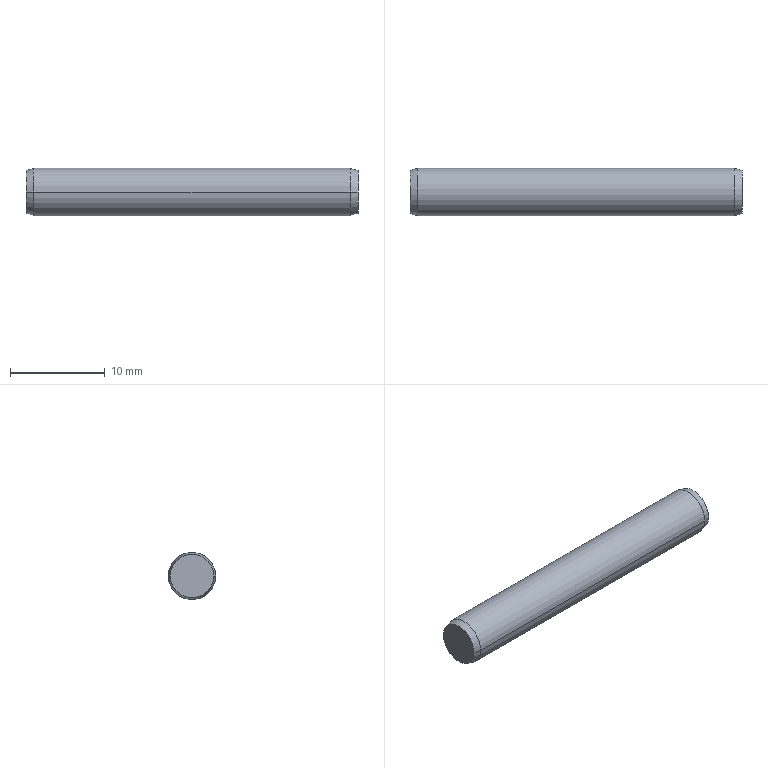Part | STEP file | 1 solid | 8 faces | box 35 x 5 x 5 mm | volume 684.607 mm3 | cone 4 | plane 2 | cylinder 2 | commonest cylinder face diameters 5 x2
STEP:
#1=CARTESIAN_POINT('',(0.,0.,0.));
#2=DIRECTION('',(0.,0.,1.));
#3=DIRECTION('',(1.,0.,0.));
#4=AXIS2_PLACEMENT_3D('',#1,#2,#3);
#5=CARTESIAN_POINT('',(35.,2.286,0.));
#6=VERTEX_POINT('',#5);
#7=CARTESIAN_POINT('',(35.,-2.286,0.));
#8=VERTEX_POINT('',#7);
#9=CARTESIAN_POINT('',(35.,0.,0.));
#10=DIRECTION('',(-1.,0.,0.));
#11=DIRECTION('',(0.,1.,0.));
#12=AXIS2_PLACEMENT_3D('',#9,#10,#11);
#13=CIRCLE('',#12,2.286);
#14=CARTESIAN_POINT('',(35.,1.143,0.));
#15=DIRECTION('',(1.,0.,0.));
#16=DIRECTION('',(0.,1.,0.));
#17=AXIS2_PLACEMENT_3D('',#14,#15,#16);
#18=PLANE('',#17);
#19=CARTESIAN_POINT('',(1.143,0.));
#20=CARTESIAN_POINT('',(1.143,-3.959));
#21=CARTESIAN_POINT('',(-2.286,-1.979));
#22=CARTESIAN_POINT('',(-5.714,0.));
#23=CARTESIAN_POINT('',(-2.286,1.979));
#24=CARTESIAN_POINT('',(1.143,3.959));
#25=CARTESIAN_POINT('',(1.143,0.));
#26=(BOUNDED_CURVE()B_SPLINE_CURVE(2,(#19,#20,#21,#22,#23,#24,#25),.UNSPECIFIED.,.T.,.F.)B_SPLINE_CURVE_WITH_KNOTS((1,2,2,2,2,1),(-2.094,0.,2.094,4.189,6.283,8.378),.UNSPECIFIED.)CURVE()GEOMETRIC_REPRESENTATION_ITEM()RATIONAL_B_SPLINE_CURVE((1.,0.5,1.,0.5,1.,0.5,1.))REPRESENTATION_ITEM(''));
#27=(GEOMETRIC_REPRESENTATION_CONTEXT(2)PARAMETRIC_REPRESENTATION_CONTEXT()REPRESENTATION_CONTEXT('',''));
#28=DEFINITIONAL_REPRESENTATION('',(#26),#27);
#29=PCURVE('',#18,#28);
#30=CARTESIAN_POINT('',(34.6,0.,0.));
#31=DIRECTION('',(-1.,0.,0.));
#32=DIRECTION('',(0.,1.,0.));
#33=AXIS2_PLACEMENT_3D('',#30,#31,#32);
#34=CONICAL_SURFACE('',#33,2.393,0.2618);
#35=CARTESIAN_POINT('',(0.,-0.4));
#36=DIRECTION('',(1.,0.));
#37=VECTOR('',#36,1.);
#38=LINE('',#35,#37);
#39=(GEOMETRIC_REPRESENTATION_CONTEXT(2)PARAMETRIC_REPRESENTATION_CONTEXT()REPRESENTATION_CONTEXT('',''));
#40=DEFINITIONAL_REPRESENTATION('',(#38),#39);
#41=PCURVE('',#34,#40);
#42=SURFACE_CURVE('',#13,(#29,#41),.PCURVE_S1.);
#43=EDGE_CURVE('',#6,#8,#42,.T.);
#44=ORIENTED_EDGE('',*,*,#43,.F.);
#45=CARTESIAN_POINT('',(35.,0.,0.));
#46=DIRECTION('',(-1.,0.,0.));
#47=DIRECTION('',(0.,1.,0.));
#48=AXIS2_PLACEMENT_3D('',#45,#46,#47);
#49=CIRCLE('',#48,2.286);
#50=CARTESIAN_POINT('',(1.143,0.));
#51=CARTESIAN_POINT('',(1.143,-3.959));
#52=CARTESIAN_POINT('',(-2.286,-1.979));
#53=CARTESIAN_POINT('',(-5.714,0.));
#54=CARTESIAN_POINT('',(-2.286,1.979));
#55=CARTESIAN_POINT('',(1.143,3.959));
#56=CARTESIAN_POINT('',(1.143,0.));
#57=(BOUNDED_CURVE()B_SPLINE_CURVE(2,(#50,#51,#52,#53,#54,#55,#56),.UNSPECIFIED.,.T.,.F.)B_SPLINE_CURVE_WITH_KNOTS((1,2,2,2,2,1),(-2.094,0.,2.094,4.189,6.283,8.378),.UNSPECIFIED.)CURVE()GEOMETRIC_REPRESENTATION_ITEM()RATIONAL_B_SPLINE_CURVE((1.,0.5,1.,0.5,1.,0.5,1.))REPRESENTATION_ITEM(''));
#58=(GEOMETRIC_REPRESENTATION_CONTEXT(2)PARAMETRIC_REPRESENTATION_CONTEXT()REPRESENTATION_CONTEXT('',''));
#59=DEFINITIONAL_REPRESENTATION('',(#57),#58);
#60=PCURVE('',#18,#59);
#61=CARTESIAN_POINT('',(34.6,0.,0.));
#62=DIRECTION('',(-1.,0.,0.));
#63=DIRECTION('',(0.,1.,0.));
#64=AXIS2_PLACEMENT_3D('',#61,#62,#63);
#65=CONICAL_SURFACE('',#64,2.393,0.2618);
#66=CARTESIAN_POINT('',(0.,-0.4));
#67=DIRECTION('',(1.,0.));
#68=VECTOR('',#67,1.);
#69=LINE('',#66,#68);
#70=(GEOMETRIC_REPRESENTATION_CONTEXT(2)PARAMETRIC_REPRESENTATION_CONTEXT()REPRESENTATION_CONTEXT('',''));
#71=DEFINITIONAL_REPRESENTATION('',(#69),#70);
#72=PCURVE('',#65,#71);
#73=SURFACE_CURVE('',#49,(#60,#72),.PCURVE_S1.);
#74=EDGE_CURVE('',#8,#6,#73,.T.);
#75=ORIENTED_EDGE('',*,*,#74,.F.);
#76=EDGE_LOOP('',(#44,#75));
#77=FACE_BOUND('',#76,.T.);
#78=ADVANCED_FACE('',(#77),#18,.T.);
#79=CARTESIAN_POINT('',(0.,2.286,0.));
#80=VERTEX_POINT('',#79);
#81=CARTESIAN_POINT('',(0.,-2.286,0.));
#82=VERTEX_POINT('',#81);
#83=CARTESIAN_POINT('',(0.,0.,0.));
#84=DIRECTION('',(-1.,0.,0.));
#85=DIRECTION('',(0.,1.,0.));
#86=AXIS2_PLACEMENT_3D('',#83,#84,#85);
#87=CIRCLE('',#86,2.286);
#88=CARTESIAN_POINT('',(0.,1.143,0.));
#89=DIRECTION('',(-1.,0.,0.));
#90=DIRECTION('',(0.,0.,1.));
#91=AXIS2_PLACEMENT_3D('',#88,#89,#90);
#92=PLANE('',#91);
#93=CARTESIAN_POINT('',(0.,-1.143));
#94=DIRECTION('',(0.,1.));
#95=AXIS2_PLACEMENT_2D('',#93,#94);
#96=CIRCLE('',#95,2.286);
#97=(GEOMETRIC_REPRESENTATION_CONTEXT(2)PARAMETRIC_REPRESENTATION_CONTEXT()REPRESENTATION_CONTEXT('',''));
#98=DEFINITIONAL_REPRESENTATION('',(#96),#97);
#99=PCURVE('',#92,#98);
#100=CARTESIAN_POINT('',(0.4,0.,0.));
#101=DIRECTION('',(1.,0.,0.));
#102=DIRECTION('',(0.,1.,0.));
#103=AXIS2_PLACEMENT_3D('',#100,#101,#102);
#104=CONICAL_SURFACE('',#103,2.393,0.2618);
#105=CARTESIAN_POINT('',(6.283,-0.4));
#106=DIRECTION('',(-1.,0.));
#107=VECTOR('',#106,1.);
#108=LINE('',#105,#107);
#109=(GEOMETRIC_REPRESENTATION_CONTEXT(2)PARAMETRIC_REPRESENTATION_CONTEXT()REPRESENTATION_CONTEXT('',''));
#110=DEFINITIONAL_REPRESENTATION('',(#108),#109);
#111=PCURVE('',#104,#110);
#112=SURFACE_CURVE('',#87,(#99,#111),.PCURVE_S1.);
#113=EDGE_CURVE('',#80,#82,#112,.T.);
#114=ORIENTED_EDGE('',*,*,#113,.T.);
#115=CARTESIAN_POINT('',(0.,0.,0.));
#116=DIRECTION('',(-1.,0.,0.));
#117=DIRECTION('',(0.,1.,0.));
#118=AXIS2_PLACEMENT_3D('',#115,#116,#117);
#119=CIRCLE('',#118,2.286);
#120=CARTESIAN_POINT('',(0.,-1.143));
#121=DIRECTION('',(0.,1.));
#122=AXIS2_PLACEMENT_2D('',#120,#121);
#123=CIRCLE('',#122,2.286);
#124=(GEOMETRIC_REPRESENTATION_CONTEXT(2)PARAMETRIC_REPRESENTATION_CONTEXT()REPRESENTATION_CONTEXT('',''));
#125=DEFINITIONAL_REPRESENTATION('',(#123),#124);
#126=PCURVE('',#92,#125);
#127=CARTESIAN_POINT('',(0.4,0.,0.));
#128=DIRECTION('',(1.,0.,0.));
#129=DIRECTION('',(0.,1.,0.));
#130=AXIS2_PLACEMENT_3D('',#127,#128,#129);
#131=CONICAL_SURFACE('',#130,2.393,0.2618);
#132=CARTESIAN_POINT('',(6.283,-0.4));
#133=DIRECTION('',(-1.,0.));
#134=VECTOR('',#133,1.);
#135=LINE('',#132,#134);
#136=(GEOMETRIC_REPRESENTATION_CONTEXT(2)PARAMETRIC_REPRESENTATION_CONTEXT()REPRESENTATION_CONTEXT('',''));
#137=DEFINITIONAL_REPRESENTATION('',(#135),#136);
#138=PCURVE('',#131,#137);
#139=SURFACE_CURVE('',#119,(#126,#138),.PCURVE_S1.);
#140=EDGE_CURVE('',#82,#80,#139,.T.);
#141=ORIENTED_EDGE('',*,*,#140,.T.);
#142=EDGE_LOOP('',(#114,#141));
#143=FACE_BOUND('',#142,.T.);
#144=ADVANCED_FACE('',(#143),#92,.T.);
#145=CARTESIAN_POINT('',(0.8,2.5,0.));
#146=VERTEX_POINT('',#145);
#147=CARTESIAN_POINT('',(0.,2.286,0.));
#148=DIRECTION('',(0.9659,0.2588,0.));
#149=VECTOR('',#148,1.);
#150=LINE('',#147,#149);
#151=CARTESIAN_POINT('',(6.283,-0.4));
#152=DIRECTION('',(0.,1.));
#153=VECTOR('',#152,1.);
#154=LINE('',#151,#153);
#155=(GEOMETRIC_REPRESENTATION_CONTEXT(2)PARAMETRIC_REPRESENTATION_CONTEXT()REPRESENTATION_CONTEXT('',''));
#156=DEFINITIONAL_REPRESENTATION('',(#154),#155);
#157=PCURVE('',#104,#156);
#158=CARTESIAN_POINT('',(0.,-0.4));
#159=DIRECTION('',(0.,1.));
#160=VECTOR('',#159,1.);
#161=LINE('',#158,#160);
#162=(GEOMETRIC_REPRESENTATION_CONTEXT(2)PARAMETRIC_REPRESENTATION_CONTEXT()REPRESENTATION_CONTEXT('',''));
#163=DEFINITIONAL_REPRESENTATION('',(#161),#162);
#164=PCURVE('',#131,#163);
#165=SURFACE_CURVE('',#150,(#157,#164),.PCURVE_S1.);
#166=EDGE_CURVE('',#80,#146,#165,.T.);
#167=ORIENTED_EDGE('',*,*,#166,.T.);
#168=CARTESIAN_POINT('',(0.8,-2.5,0.));
#169=VERTEX_POINT('',#168);
#170=CARTESIAN_POINT('',(0.8,0.,0.));
#171=DIRECTION('',(-1.,0.,0.));
#172=DIRECTION('',(0.,1.,0.));
#173=AXIS2_PLACEMENT_3D('',#170,#171,#172);
#174=CIRCLE('',#173,2.5);
#175=CARTESIAN_POINT('',(6.283,0.4));
#176=DIRECTION('',(-1.,0.));
#177=VECTOR('',#176,1.);
#178=LINE('',#175,#177);
#179=(GEOMETRIC_REPRESENTATION_CONTEXT(2)PARAMETRIC_REPRESENTATION_CONTEXT()REPRESENTATION_CONTEXT('',''));
#180=DEFINITIONAL_REPRESENTATION('',(#178),#179);
#181=PCURVE('',#104,#180);
#182=CARTESIAN_POINT('',(17.5,0.,0.));
#183=DIRECTION('',(-1.,0.,0.));
#184=DIRECTION('',(0.,1.,0.));
#185=AXIS2_PLACEMENT_3D('',#182,#183,#184);
#186=CYLINDRICAL_SURFACE('',#185,2.5);
#187=CARTESIAN_POINT('',(0.,16.7));
#188=DIRECTION('',(1.,0.));
#189=VECTOR('',#188,1.);
#190=LINE('',#187,#189);
#191=(GEOMETRIC_REPRESENTATION_CONTEXT(2)PARAMETRIC_REPRESENTATION_CONTEXT()REPRESENTATION_CONTEXT('',''));
#192=DEFINITIONAL_REPRESENTATION('',(#190),#191);
#193=PCURVE('',#186,#192);
#194=SURFACE_CURVE('',#174,(#181,#193),.PCURVE_S1.);
#195=EDGE_CURVE('',#146,#169,#194,.T.);
#196=ORIENTED_EDGE('',*,*,#195,.T.);
#197=CARTESIAN_POINT('',(0.,-2.286,0.));
#198=DIRECTION('',(0.9659,-0.2588,0.));
#199=VECTOR('',#198,1.);
#200=LINE('',#197,#199);
#201=CARTESIAN_POINT('',(3.142,-0.4));
#202=DIRECTION('',(0.,1.));
#203=VECTOR('',#202,1.);
#204=LINE('',#201,#203);
#205=(GEOMETRIC_REPRESENTATION_CONTEXT(2)PARAMETRIC_REPRESENTATION_CONTEXT()REPRESENTATION_CONTEXT('',''));
#206=DEFINITIONAL_REPRESENTATION('',(#204),#205);
#207=PCURVE('',#104,#206);
#208=CARTESIAN_POINT('',(3.142,-0.4));
#209=DIRECTION('',(0.,1.));
#210=VECTOR('',#209,1.);
#211=LINE('',#208,#210);
#212=(GEOMETRIC_REPRESENTATION_CONTEXT(2)PARAMETRIC_REPRESENTATION_CONTEXT()REPRESENTATION_CONTEXT('',''));
#213=DEFINITIONAL_REPRESENTATION('',(#211),#212);
#214=PCURVE('',#131,#213);
#215=SURFACE_CURVE('',#200,(#207,#214),.PCURVE_S1.);
#216=EDGE_CURVE('',#82,#169,#215,.T.);
#217=ORIENTED_EDGE('',*,*,#216,.F.);
#218=ORIENTED_EDGE('',*,*,#113,.F.);
#219=EDGE_LOOP('',(#167,#196,#217,#218));
#220=FACE_BOUND('',#219,.T.);
#221=ADVANCED_FACE('',(#220),#104,.T.);
#222=CARTESIAN_POINT('',(34.2,2.5,0.));
#223=VERTEX_POINT('',#222);
#224=CARTESIAN_POINT('',(0.8,2.5,0.));
#225=DIRECTION('',(1.,0.,0.));
#226=VECTOR('',#225,1.);
#227=LINE('',#224,#226);
#228=CARTESIAN_POINT('',(0.,16.7));
#229=DIRECTION('',(0.,-1.));
#230=VECTOR('',#229,1.);
#231=LINE('',#228,#230);
#232=(GEOMETRIC_REPRESENTATION_CONTEXT(2)PARAMETRIC_REPRESENTATION_CONTEXT()REPRESENTATION_CONTEXT('',''));
#233=DEFINITIONAL_REPRESENTATION('',(#231),#232);
#234=PCURVE('',#186,#233);
#235=CARTESIAN_POINT('',(17.5,0.,0.));
#236=DIRECTION('',(-1.,0.,0.));
#237=DIRECTION('',(0.,1.,0.));
#238=AXIS2_PLACEMENT_3D('',#235,#236,#237);
#239=CYLINDRICAL_SURFACE('',#238,2.5);
#240=CARTESIAN_POINT('',(6.283,16.7));
#241=DIRECTION('',(0.,-1.));
#242=VECTOR('',#241,1.);
#243=LINE('',#240,#242);
#244=(GEOMETRIC_REPRESENTATION_CONTEXT(2)PARAMETRIC_REPRESENTATION_CONTEXT()REPRESENTATION_CONTEXT('',''));
#245=DEFINITIONAL_REPRESENTATION('',(#243),#244);
#246=PCURVE('',#239,#245);
#247=SURFACE_CURVE('',#227,(#234,#246),.PCURVE_S1.);
#248=EDGE_CURVE('',#146,#223,#247,.T.);
#249=ORIENTED_EDGE('',*,*,#248,.T.);
#250=CARTESIAN_POINT('',(34.2,-2.5,0.));
#251=VERTEX_POINT('',#250);
#252=CARTESIAN_POINT('',(34.2,0.,0.));
#253=DIRECTION('',(-1.,0.,0.));
#254=DIRECTION('',(0.,1.,0.));
#255=AXIS2_PLACEMENT_3D('',#252,#253,#254);
#256=CIRCLE('',#255,2.5);
#257=CARTESIAN_POINT('',(0.,-16.7));
#258=DIRECTION('',(1.,0.));
#259=VECTOR('',#258,1.);
#260=LINE('',#257,#259);
#261=(GEOMETRIC_REPRESENTATION_CONTEXT(2)PARAMETRIC_REPRESENTATION_CONTEXT()REPRESENTATION_CONTEXT('',''));
#262=DEFINITIONAL_REPRESENTATION('',(#260),#261);
#263=PCURVE('',#186,#262);
#264=CARTESIAN_POINT('',(0.,0.4));
#265=DIRECTION('',(1.,0.));
#266=VECTOR('',#265,1.);
#267=LINE('',#264,#266);
#268=(GEOMETRIC_REPRESENTATION_CONTEXT(2)PARAMETRIC_REPRESENTATION_CONTEXT()REPRESENTATION_CONTEXT('',''));
#269=DEFINITIONAL_REPRESENTATION('',(#267),#268);
#270=PCURVE('',#34,#269);
#271=SURFACE_CURVE('',#256,(#263,#270),.PCURVE_S1.);
#272=EDGE_CURVE('',#223,#251,#271,.T.);
#273=ORIENTED_EDGE('',*,*,#272,.T.);
#274=CARTESIAN_POINT('',(0.8,-2.5,0.));
#275=DIRECTION('',(1.,0.,0.));
#276=VECTOR('',#275,1.);
#277=LINE('',#274,#276);
#278=CARTESIAN_POINT('',(3.142,16.7));
#279=DIRECTION('',(0.,-1.));
#280=VECTOR('',#279,1.);
#281=LINE('',#278,#280);
#282=(GEOMETRIC_REPRESENTATION_CONTEXT(2)PARAMETRIC_REPRESENTATION_CONTEXT()REPRESENTATION_CONTEXT('',''));
#283=DEFINITIONAL_REPRESENTATION('',(#281),#282);
#284=PCURVE('',#186,#283);
#285=CARTESIAN_POINT('',(3.142,16.7));
#286=DIRECTION('',(0.,-1.));
#287=VECTOR('',#286,1.);
#288=LINE('',#285,#287);
#289=(GEOMETRIC_REPRESENTATION_CONTEXT(2)PARAMETRIC_REPRESENTATION_CONTEXT()REPRESENTATION_CONTEXT('',''));
#290=DEFINITIONAL_REPRESENTATION('',(#288),#289);
#291=PCURVE('',#239,#290);
#292=SURFACE_CURVE('',#277,(#284,#291),.PCURVE_S1.);
#293=EDGE_CURVE('',#169,#251,#292,.T.);
#294=ORIENTED_EDGE('',*,*,#293,.F.);
#295=ORIENTED_EDGE('',*,*,#195,.F.);
#296=EDGE_LOOP('',(#249,#273,#294,#295));
#297=FACE_BOUND('',#296,.T.);
#298=ADVANCED_FACE('',(#297),#186,.T.);
#299=CARTESIAN_POINT('',(34.2,2.5,0.));
#300=DIRECTION('',(0.9659,-0.2588,0.));
#301=VECTOR('',#300,1.);
#302=LINE('',#299,#301);
#303=CARTESIAN_POINT('',(0.,0.4));
#304=DIRECTION('',(0.,-1.));
#305=VECTOR('',#304,1.);
#306=LINE('',#303,#305);
#307=(GEOMETRIC_REPRESENTATION_CONTEXT(2)PARAMETRIC_REPRESENTATION_CONTEXT()REPRESENTATION_CONTEXT('',''));
#308=DEFINITIONAL_REPRESENTATION('',(#306),#307);
#309=PCURVE('',#34,#308);
#310=CARTESIAN_POINT('',(6.283,0.4));
#311=DIRECTION('',(0.,-1.));
#312=VECTOR('',#311,1.);
#313=LINE('',#310,#312);
#314=(GEOMETRIC_REPRESENTATION_CONTEXT(2)PARAMETRIC_REPRESENTATION_CONTEXT()REPRESENTATION_CONTEXT('',''));
#315=DEFINITIONAL_REPRESENTATION('',(#313),#314);
#316=PCURVE('',#65,#315);
#317=SURFACE_CURVE('',#302,(#309,#316),.PCURVE_S1.);
#318=EDGE_CURVE('',#223,#6,#317,.T.);
#319=ORIENTED_EDGE('',*,*,#318,.T.);
#320=ORIENTED_EDGE('',*,*,#43,.T.);
#321=CARTESIAN_POINT('',(34.2,-2.5,0.));
#322=DIRECTION('',(0.9659,0.2588,0.));
#323=VECTOR('',#322,1.);
#324=LINE('',#321,#323);
#325=CARTESIAN_POINT('',(3.142,0.4));
#326=DIRECTION('',(0.,-1.));
#327=VECTOR('',#326,1.);
#328=LINE('',#325,#327);
#329=(GEOMETRIC_REPRESENTATION_CONTEXT(2)PARAMETRIC_REPRESENTATION_CONTEXT()REPRESENTATION_CONTEXT('',''));
#330=DEFINITIONAL_REPRESENTATION('',(#328),#329);
#331=PCURVE('',#34,#330);
#332=CARTESIAN_POINT('',(3.142,0.4));
#333=DIRECTION('',(0.,-1.));
#334=VECTOR('',#333,1.);
#335=LINE('',#332,#334);
#336=(GEOMETRIC_REPRESENTATION_CONTEXT(2)PARAMETRIC_REPRESENTATION_CONTEXT()REPRESENTATION_CONTEXT('',''));
#337=DEFINITIONAL_REPRESENTATION('',(#335),#336);
#338=PCURVE('',#65,#337);
#339=SURFACE_CURVE('',#324,(#331,#338),.PCURVE_S1.);
#340=EDGE_CURVE('',#251,#8,#339,.T.);
#341=ORIENTED_EDGE('',*,*,#340,.F.);
#342=ORIENTED_EDGE('',*,*,#272,.F.);
#343=EDGE_LOOP('',(#319,#320,#341,#342));
#344=FACE_BOUND('',#343,.T.);
#345=ADVANCED_FACE('',(#344),#34,.T.);
#346=ORIENTED_EDGE('',*,*,#318,.F.);
#347=CARTESIAN_POINT('',(34.2,0.,0.));
#348=DIRECTION('',(-1.,0.,0.));
#349=DIRECTION('',(0.,1.,0.));
#350=AXIS2_PLACEMENT_3D('',#347,#348,#349);
#351=CIRCLE('',#350,2.5);
#352=CARTESIAN_POINT('',(0.,0.4));
#353=DIRECTION('',(1.,0.));
#354=VECTOR('',#353,1.);
#355=LINE('',#352,#354);
#356=(GEOMETRIC_REPRESENTATION_CONTEXT(2)PARAMETRIC_REPRESENTATION_CONTEXT()REPRESENTATION_CONTEXT('',''));
#357=DEFINITIONAL_REPRESENTATION('',(#355),#356);
#358=PCURVE('',#65,#357);
#359=CARTESIAN_POINT('',(0.,-16.7));
#360=DIRECTION('',(1.,0.));
#361=VECTOR('',#360,1.);
#362=LINE('',#359,#361);
#363=(GEOMETRIC_REPRESENTATION_CONTEXT(2)PARAMETRIC_REPRESENTATION_CONTEXT()REPRESENTATION_CONTEXT('',''));
#364=DEFINITIONAL_REPRESENTATION('',(#362),#363);
#365=PCURVE('',#239,#364);
#366=SURFACE_CURVE('',#351,(#358,#365),.PCURVE_S1.);
#367=EDGE_CURVE('',#251,#223,#366,.T.);
#368=ORIENTED_EDGE('',*,*,#367,.F.);
#369=ORIENTED_EDGE('',*,*,#340,.T.);
#370=ORIENTED_EDGE('',*,*,#74,.T.);
#371=EDGE_LOOP('',(#346,#368,#369,#370));
#372=FACE_BOUND('',#371,.T.);
#373=ADVANCED_FACE('',(#372),#65,.T.);
#374=ORIENTED_EDGE('',*,*,#248,.F.);
#375=CARTESIAN_POINT('',(0.8,0.,0.));
#376=DIRECTION('',(-1.,0.,0.));
#377=DIRECTION('',(0.,1.,0.));
#378=AXIS2_PLACEMENT_3D('',#375,#376,#377);
#379=CIRCLE('',#378,2.5);
#380=CARTESIAN_POINT('',(0.,16.7));
#381=DIRECTION('',(1.,0.));
#382=VECTOR('',#381,1.);
#383=LINE('',#380,#382);
#384=(GEOMETRIC_REPRESENTATION_CONTEXT(2)PARAMETRIC_REPRESENTATION_CONTEXT()REPRESENTATION_CONTEXT('',''));
#385=DEFINITIONAL_REPRESENTATION('',(#383),#384);
#386=PCURVE('',#239,#385);
#387=CARTESIAN_POINT('',(6.283,0.4));
#388=DIRECTION('',(-1.,0.));
#389=VECTOR('',#388,1.);
#390=LINE('',#387,#389);
#391=(GEOMETRIC_REPRESENTATION_CONTEXT(2)PARAMETRIC_REPRESENTATION_CONTEXT()REPRESENTATION_CONTEXT('',''));
#392=DEFINITIONAL_REPRESENTATION('',(#390),#391);
#393=PCURVE('',#131,#392);
#394=SURFACE_CURVE('',#379,(#386,#393),.PCURVE_S1.);
#395=EDGE_CURVE('',#169,#146,#394,.T.);
#396=ORIENTED_EDGE('',*,*,#395,.F.);
#397=ORIENTED_EDGE('',*,*,#293,.T.);
#398=ORIENTED_EDGE('',*,*,#367,.T.);
#399=EDGE_LOOP('',(#374,#396,#397,#398));
#400=FACE_BOUND('',#399,.T.);
#401=ADVANCED_FACE('',(#400),#239,.T.);
#402=ORIENTED_EDGE('',*,*,#166,.F.);
#403=ORIENTED_EDGE('',*,*,#140,.F.);
#404=ORIENTED_EDGE('',*,*,#216,.T.);
#405=ORIENTED_EDGE('',*,*,#395,.T.);
#406=EDGE_LOOP('',(#402,#403,#404,#405));
#407=FACE_BOUND('',#406,.T.);
#408=ADVANCED_FACE('',(#407),#131,.T.);
#409=CLOSED_SHELL('',(#78,#144,#221,#298,#345,#373,#401,#408));
#410=MANIFOLD_SOLID_BREP('',#409);
#411=(LENGTH_UNIT()NAMED_UNIT(*)SI_UNIT(.MILLI.,.METRE.));
#412=UNCERTAINTY_MEASURE_WITH_UNIT(LENGTH_MEASURE(0.0000001),#411,'','');
#413=(NAMED_UNIT(*)PLANE_ANGLE_UNIT()SI_UNIT($,.RADIAN.));
#414=(NAMED_UNIT(*)SI_UNIT($,.STERADIAN.)SOLID_ANGLE_UNIT());
#415=(GEOMETRIC_REPRESENTATION_CONTEXT(3)GLOBAL_UNCERTAINTY_ASSIGNED_CONTEXT((#412))GLOBAL_UNIT_ASSIGNED_CONTEXT((#411,#413,#414))REPRESENTATION_CONTEXT('',''));
#416=ADVANCED_BREP_SHAPE_REPRESENTATION('',(#4,#410),#415);